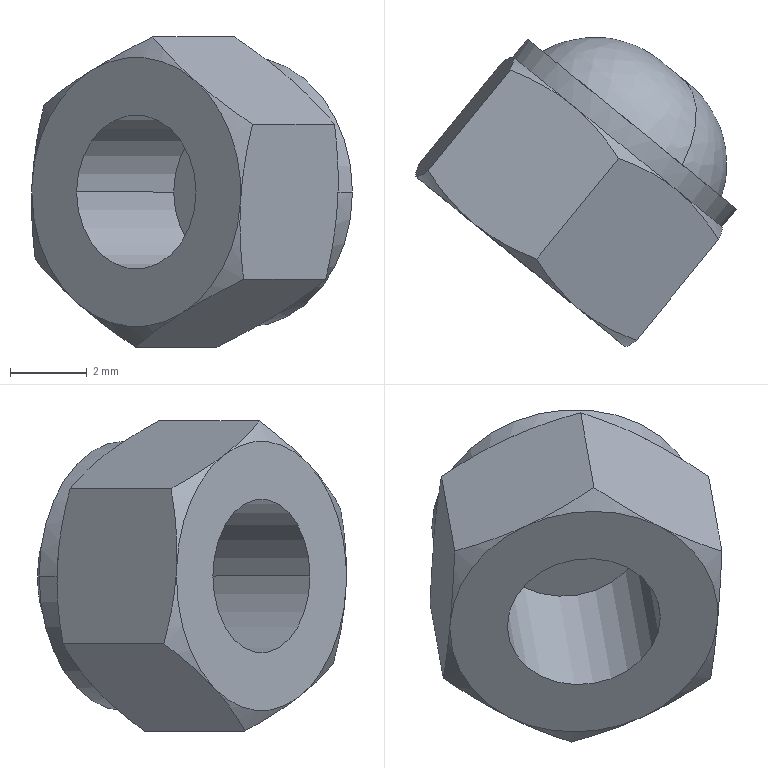Part | SolidWorks | features BaseBody 1 | 1 solid | 29 faces | box 8.341 x 8.038 x 8.061 mm | volume 172.858 mm3 | cone 14 | plane 9 | cylinder 4 | spline 2 | commonest cylinder face diameters 4 x2 7 x2
STEP:
#1=CARTESIAN_POINT('',(537.312,-141.656,258.325));
#2=VERTEX_POINT('',#1);
#3=CARTESIAN_POINT('',(534.695,-139.529,253.362));
#4=VERTEX_POINT('',#3);
#5=CARTESIAN_POINT('',(536.004,-140.592,255.843));
#6=DIRECTION('',(-0.6309,-0.7758,0.000000012));
#7=DIRECTION('',(0.7758,-0.6309,0.));
#8=AXIS2_PLACEMENT_3D('',#5,#6,#7);
#9=CIRCLE('',#8,3.);
#10=EDGE_CURVE('',#2,#4,#9,.T.);
#11=ORIENTED_EDGE('',*,*,#10,.F.);
#12=CARTESIAN_POINT('',(537.076,-139.274,255.843));
#13=VERTEX_POINT('',#12);
#14=CARTESIAN_POINT('',(535.614,-141.5,256.24));
#15=DIRECTION('',(-0.6417,0.5218,0.5621));
#16=DIRECTION('',(0.4361,-0.3546,0.8271));
#17=AXIS2_PLACEMENT_3D('',#14,#15,#16);
#18=CIRCLE('',#17,2.693);
#19=EDGE_CURVE('',#2,#13,#18,.T.);
#20=ORIENTED_EDGE('',*,*,#19,.T.);
#21=CARTESIAN_POINT('',(535.195,-141.159,255.446));
#22=DIRECTION('',(0.6417,-0.5218,-0.5621));
#23=DIRECTION('',(-0.4361,0.3546,-0.8271));
#24=AXIS2_PLACEMENT_3D('',#21,#22,#23);
#25=CIRCLE('',#24,2.693);
#26=EDGE_CURVE('',#4,#13,#25,.T.);
#27=ORIENTED_EDGE('',*,*,#26,.F.);
#28=EDGE_LOOP('',(#11,#20,#27));
#29=FACE_OUTER_BOUND('',#28,.T.);
#30=CARTESIAN_POINT('',(537.312,-141.656,258.325));
#31=CARTESIAN_POINT('',(533.462,-138.525,261.697));
#32=CARTESIAN_POINT('',(530.845,-136.398,256.735));
#33=CARTESIAN_POINT('',(534.695,-139.529,253.362));
#34=CARTESIAN_POINT('',(537.905,-140.499,257.928));
#35=CARTESIAN_POINT('',(534.671,-137.869,260.761));
#36=CARTESIAN_POINT('',(532.473,-136.081,256.592));
#37=CARTESIAN_POINT('',(535.707,-138.712,253.759));
#38=CARTESIAN_POINT('',(537.813,-139.56,256.95));
#39=CARTESIAN_POINT('',(536.096,-138.164,258.453));
#40=CARTESIAN_POINT('',(534.929,-137.215,256.241));
#41=CARTESIAN_POINT('',(536.646,-138.611,254.737));
#42=CARTESIAN_POINT('',(537.076,-139.274,255.843));
#43=CARTESIAN_POINT('',(537.076,-139.274,255.843));
#44=CARTESIAN_POINT('',(537.076,-139.274,255.843));
#45=CARTESIAN_POINT('',(537.076,-139.274,255.843));
#46=(BOUNDED_SURFACE()B_SPLINE_SURFACE(3,3,((#30,#31,#32,#33),(#34,#35,#36,#37),(#38,#39,#40,#41),(#42,#43,#44,#45)),.UNSPECIFIED.,.F.,.F.,.F.)B_SPLINE_SURFACE_WITH_KNOTS((4,4),(4,4),(0.,1.),(0.,1.),.UNSPECIFIED.)GEOMETRIC_REPRESENTATION_ITEM()RATIONAL_B_SPLINE_SURFACE(((1.,0.3333,0.3333,1.),(0.8455,0.2818,0.2818,0.8455),(0.8455,0.2818,0.2818,0.8455),(1.,0.3333,0.3333,1.)))REPRESENTATION_ITEM('')SURFACE());
#47=ADVANCED_FACE('',(#29),#46,.T.);
#48=CARTESIAN_POINT('',(534.074,-139.796,255.843));
#49=VERTEX_POINT('',#48);
#50=CARTESIAN_POINT('',(537.177,-142.32,255.843));
#51=VERTEX_POINT('',#50);
#52=CARTESIAN_POINT('',(535.625,-141.058,255.843));
#53=DIRECTION('',(-0.6309,-0.7758,0.000000012));
#54=DIRECTION('',(0.7758,-0.6309,0.));
#55=AXIS2_PLACEMENT_3D('',#52,#53,#54);
#56=CIRCLE('',#55,2.);
#57=EDGE_CURVE('',#49,#51,#56,.T.);
#58=ORIENTED_EDGE('',*,*,#57,.F.);
#59=CARTESIAN_POINT('',(531.55,-142.899,255.843));
#60=VERTEX_POINT('',#59);
#61=CARTESIAN_POINT('',(531.55,-142.899,255.843));
#62=DIRECTION('',(-0.6309,-0.7758,0.000000012));
#63=VECTOR('',#62,1000.);
#64=LINE('',#61,#63);
#65=EDGE_CURVE('',#49,#60,#64,.T.);
#66=ORIENTED_EDGE('',*,*,#65,.T.);
#67=CARTESIAN_POINT('',(534.653,-145.423,255.843));
#68=VERTEX_POINT('',#67);
#69=CARTESIAN_POINT('',(533.101,-144.161,255.843));
#70=DIRECTION('',(-0.6309,-0.7758,0.000000012));
#71=DIRECTION('',(0.7758,-0.6309,0.));
#72=AXIS2_PLACEMENT_3D('',#69,#70,#71);
#73=CIRCLE('',#72,2.);
#74=EDGE_CURVE('',#60,#68,#73,.T.);
#75=ORIENTED_EDGE('',*,*,#74,.T.);
#76=CARTESIAN_POINT('',(534.653,-145.423,255.843));
#77=DIRECTION('',(-0.6309,-0.7758,0.000000012));
#78=VECTOR('',#77,1000.);
#79=LINE('',#76,#78);
#80=EDGE_CURVE('',#51,#68,#79,.T.);
#81=ORIENTED_EDGE('',*,*,#80,.F.);
#82=EDGE_LOOP('',(#58,#66,#75,#81));
#83=FACE_OUTER_BOUND('',#82,.T.);
#84=CARTESIAN_POINT('',(533.101,-144.161,255.843));
#85=DIRECTION('',(-0.6309,-0.7758,0.000000012));
#86=DIRECTION('',(0.7758,-0.6309,0.));
#87=AXIS2_PLACEMENT_3D('',#84,#85,#86);
#88=CYLINDRICAL_SURFACE('',#87,2.);
#89=ADVANCED_FACE('',(#83),#88,.F.);
#90=CARTESIAN_POINT('',(531.575,-142.92,252.949));
#91=VERTEX_POINT('',#90);
#92=CARTESIAN_POINT('',(530.386,-141.953,255.843));
#93=VERTEX_POINT('',#92);
#94=CARTESIAN_POINT('',(533.101,-144.161,255.843));
#95=DIRECTION('',(0.6309,0.7758,-0.000000012));
#96=DIRECTION('',(-0.7758,0.6309,0.));
#97=AXIS2_PLACEMENT_3D('',#94,#95,#96);
#98=CIRCLE('',#97,3.5);
#99=EDGE_CURVE('',#91,#93,#98,.T.);
#100=ORIENTED_EDGE('',*,*,#99,.T.);
#101=CARTESIAN_POINT('',(530.382,-141.943,255.843));
#102=VERTEX_POINT('',#101);
#103=CARTESIAN_POINT('',(530.162,-141.365,255.843));
#104=DIRECTION('',(-0.3564,0.9343,-0.000000006));
#105=VECTOR('',#104,1000.);
#106=LINE('',#103,#105);
#107=EDGE_CURVE('',#93,#102,#106,.T.);
#108=ORIENTED_EDGE('',*,*,#107,.T.);
#109=CARTESIAN_POINT('',(530.476,-141.623,254.084));
#110=VERTEX_POINT('',#109);
#111=CARTESIAN_POINT('',(530.382,-141.943,255.843));
#112=CARTESIAN_POINT('',(530.364,-141.895,255.245));
#113=CARTESIAN_POINT('',(530.403,-141.779,254.661));
#114=CARTESIAN_POINT('',(530.476,-141.623,254.084));
#115=B_SPLINE_CURVE_WITH_KNOTS('',3,(#111,#112,#113,#114),.UNSPECIFIED.,.F.,.F.,(4,4),(0.0002548,0.002045),.UNSPECIFIED.);
#116=EDGE_CURVE('',#102,#110,#115,.T.);
#117=ORIENTED_EDGE('',*,*,#116,.T.);
#118=CARTESIAN_POINT('',(530.476,-141.623,254.084));
#119=CARTESIAN_POINT('',(530.779,-142.115,253.713));
#120=CARTESIAN_POINT('',(531.133,-142.56,253.336));
#121=CARTESIAN_POINT('',(531.575,-142.92,252.949));
#122=B_SPLINE_CURVE_WITH_KNOTS('',3,(#118,#119,#120,#121),.UNSPECIFIED.,.F.,.F.,(4,4),(0.,0.002045),.UNSPECIFIED.);
#123=EDGE_CURVE('',#110,#91,#122,.T.);
#124=ORIENTED_EDGE('',*,*,#123,.T.);
#125=EDGE_LOOP('',(#100,#108,#117,#124));
#126=FACE_OUTER_BOUND('',#125,.T.);
#127=CARTESIAN_POINT('',(533.3,-143.917,255.843));
#128=DIRECTION('',(0.6309,0.7758,-0.000000012));
#129=DIRECTION('',(-0.7758,0.6309,0.));
#130=AXIS2_PLACEMENT_3D('',#127,#128,#129);
#131=CONICAL_SURFACE('',#130,4.045,1.047);
#132=ADVANCED_FACE('',(#126),#131,.T.);
#133=CARTESIAN_POINT('',(538.333,-143.26,255.587));
#134=VERTEX_POINT('',#133);
#135=CARTESIAN_POINT('',(538.341,-143.266,255.843));
#136=VERTEX_POINT('',#135);
#137=CARTESIAN_POINT('',(535.625,-141.058,255.843));
#138=DIRECTION('',(-0.6309,-0.7758,0.000000012));
#139=DIRECTION('',(-0.4361,0.3546,-0.8271));
#140=AXIS2_PLACEMENT_3D('',#137,#138,#139);
#141=CIRCLE('',#140,3.5);
#142=EDGE_CURVE('',#134,#136,#141,.T.);
#143=ORIENTED_EDGE('',*,*,#142,.T.);
#144=CARTESIAN_POINT('',(538.344,-143.276,255.843));
#145=VERTEX_POINT('',#144);
#146=CARTESIAN_POINT('',(538.565,-143.854,255.843));
#147=DIRECTION('',(0.3564,-0.9343,0.000000006));
#148=VECTOR('',#147,1000.);
#149=LINE('',#146,#148);
#150=EDGE_CURVE('',#136,#145,#149,.T.);
#151=ORIENTED_EDGE('',*,*,#150,.T.);
#152=CARTESIAN_POINT('',(538.333,-143.26,255.587));
#153=CARTESIAN_POINT('',(538.338,-143.264,255.673));
#154=CARTESIAN_POINT('',(538.342,-143.27,255.758));
#155=CARTESIAN_POINT('',(538.344,-143.276,255.843));
#156=B_SPLINE_CURVE_WITH_KNOTS('',3,(#152,#153,#154,#155),.UNSPECIFIED.,.F.,.F.,(4,4),(0.,0.0002548),.UNSPECIFIED.);
#157=EDGE_CURVE('',#134,#145,#156,.T.);
#158=ORIENTED_EDGE('',*,*,#157,.F.);
#159=EDGE_LOOP('',(#143,#151,#158));
#160=FACE_OUTER_BOUND('',#159,.T.);
#161=CARTESIAN_POINT('',(535.427,-141.302,255.843));
#162=DIRECTION('',(-0.6309,-0.7758,0.000000012));
#163=DIRECTION('',(0.7758,-0.6309,0.));
#164=AXIS2_PLACEMENT_3D('',#161,#162,#163);
#165=CONICAL_SURFACE('',#164,4.045,1.047);
#166=ADVANCED_FACE('',(#160),#165,.T.);
#167=CARTESIAN_POINT('',(538.719,-142.801,255.843));
#168=VERTEX_POINT('',#167);
#169=CARTESIAN_POINT('',(533.288,-138.384,255.843));
#170=VERTEX_POINT('',#169);
#171=CARTESIAN_POINT('',(536.004,-140.592,255.843));
#172=DIRECTION('',(-0.6309,-0.7758,0.000000012));
#173=DIRECTION('',(0.7758,-0.6309,0.));
#174=AXIS2_PLACEMENT_3D('',#171,#172,#173);
#175=CIRCLE('',#174,3.5);
#176=EDGE_CURVE('',#168,#170,#175,.T.);
#177=ORIENTED_EDGE('',*,*,#176,.T.);
#178=CARTESIAN_POINT('',(532.91,-138.85,255.843));
#179=VERTEX_POINT('',#178);
#180=CARTESIAN_POINT('',(533.099,-138.617,255.843));
#181=DIRECTION('',(-0.6309,-0.7758,0.000000012));
#182=VECTOR('',#181,1000.);
#183=LINE('',#180,#182);
#184=EDGE_CURVE('',#170,#179,#183,.T.);
#185=ORIENTED_EDGE('',*,*,#184,.T.);
#186=CARTESIAN_POINT('',(532.917,-138.856,256.1));
#187=VERTEX_POINT('',#186);
#188=CARTESIAN_POINT('',(535.625,-141.058,255.843));
#189=DIRECTION('',(-0.6309,-0.7758,0.000000012));
#190=DIRECTION('',(-0.4361,0.3546,-0.8271));
#191=AXIS2_PLACEMENT_3D('',#188,#189,#190);
#192=CIRCLE('',#191,3.5);
#193=EDGE_CURVE('',#187,#179,#192,.T.);
#194=ORIENTED_EDGE('',*,*,#193,.F.);
#195=CARTESIAN_POINT('',(534.443,-140.097,258.994));
#196=VERTEX_POINT('',#195);
#197=CARTESIAN_POINT('',(535.625,-141.058,255.843));
#198=DIRECTION('',(-0.6309,-0.7758,0.000000012));
#199=DIRECTION('',(-0.4361,0.3546,-0.8271));
#200=AXIS2_PLACEMENT_3D('',#197,#198,#199);
#201=CIRCLE('',#200,3.5);
#202=EDGE_CURVE('',#196,#187,#201,.T.);
#203=ORIENTED_EDGE('',*,*,#202,.F.);
#204=CARTESIAN_POINT('',(537.151,-142.299,258.738));
#205=VERTEX_POINT('',#204);
#206=CARTESIAN_POINT('',(535.625,-141.058,255.843));
#207=DIRECTION('',(-0.6309,-0.7758,0.000000012));
#208=DIRECTION('',(-0.4361,0.3546,-0.8271));
#209=AXIS2_PLACEMENT_3D('',#206,#207,#208);
#210=CIRCLE('',#209,3.5);
#211=EDGE_CURVE('',#205,#196,#210,.T.);
#212=ORIENTED_EDGE('',*,*,#211,.F.);
#213=CARTESIAN_POINT('',(535.625,-141.058,255.843));
#214=DIRECTION('',(-0.6309,-0.7758,0.000000012));
#215=DIRECTION('',(-0.4361,0.3546,-0.8271));
#216=AXIS2_PLACEMENT_3D('',#213,#214,#215);
#217=CIRCLE('',#216,3.5);
#218=EDGE_CURVE('',#136,#205,#217,.T.);
#219=ORIENTED_EDGE('',*,*,#218,.F.);
#220=CARTESIAN_POINT('',(538.53,-143.033,255.843));
#221=DIRECTION('',(-0.6309,-0.7758,0.000000012));
#222=VECTOR('',#221,1000.);
#223=LINE('',#220,#222);
#224=EDGE_CURVE('',#168,#136,#223,.T.);
#225=ORIENTED_EDGE('',*,*,#224,.F.);
#226=EDGE_LOOP('',(#177,#185,#194,#203,#212,#219,#225));
#227=FACE_OUTER_BOUND('',#226,.T.);
#228=CARTESIAN_POINT('',(535.814,-140.825,255.843));
#229=DIRECTION('',(-0.6309,-0.7758,0.000000012));
#230=DIRECTION('',(0.7758,-0.6309,0.));
#231=AXIS2_PLACEMENT_3D('',#228,#229,#230);
#232=CYLINDRICAL_SURFACE('',#231,3.5);
#233=ADVANCED_FACE('',(#227),#232,.T.);
#234=CARTESIAN_POINT('',(533.101,-144.161,255.843));
#235=DIRECTION('',(-0.6309,-0.7758,0.000000012));
#236=DIRECTION('',(0.7758,-0.6309,0.));
#237=AXIS2_PLACEMENT_3D('',#234,#235,#236);
#238=CIRCLE('',#237,2.);
#239=EDGE_CURVE('',#68,#60,#238,.T.);
#240=ORIENTED_EDGE('',*,*,#239,.F.);
#241=ORIENTED_EDGE('',*,*,#74,.F.);
#242=EDGE_LOOP('',(#240,#241));
#243=FACE_BOUND('',#242,.T.);
#244=ORIENTED_EDGE('',*,*,#99,.F.);
#245=CARTESIAN_POINT('',(534.283,-145.122,252.692));
#246=VERTEX_POINT('',#245);
#247=CARTESIAN_POINT('',(533.101,-144.161,255.843));
#248=DIRECTION('',(0.6309,0.7758,-0.000000012));
#249=DIRECTION('',(-0.7758,0.6309,0.));
#250=AXIS2_PLACEMENT_3D('',#247,#248,#249);
#251=CIRCLE('',#250,3.5);
#252=EDGE_CURVE('',#246,#91,#251,.T.);
#253=ORIENTED_EDGE('',*,*,#252,.F.);
#254=CARTESIAN_POINT('',(535.81,-146.364,255.587));
#255=VERTEX_POINT('',#254);
#256=CARTESIAN_POINT('',(533.101,-144.161,255.843));
#257=DIRECTION('',(0.6309,0.7758,-0.000000012));
#258=DIRECTION('',(-0.7758,0.6309,0.));
#259=AXIS2_PLACEMENT_3D('',#256,#257,#258);
#260=CIRCLE('',#259,3.5);
#261=EDGE_CURVE('',#255,#246,#260,.T.);
#262=ORIENTED_EDGE('',*,*,#261,.F.);
#263=CARTESIAN_POINT('',(534.628,-145.403,258.738));
#264=VERTEX_POINT('',#263);
#265=CARTESIAN_POINT('',(533.101,-144.161,255.843));
#266=DIRECTION('',(0.6309,0.7758,-0.000000012));
#267=DIRECTION('',(-0.7758,0.6309,0.));
#268=AXIS2_PLACEMENT_3D('',#265,#266,#267);
#269=CIRCLE('',#268,3.5);
#270=EDGE_CURVE('',#264,#255,#269,.T.);
#271=ORIENTED_EDGE('',*,*,#270,.F.);
#272=CARTESIAN_POINT('',(531.92,-143.2,258.994));
#273=VERTEX_POINT('',#272);
#274=CARTESIAN_POINT('',(533.101,-144.161,255.843));
#275=DIRECTION('',(0.6309,0.7758,-0.000000012));
#276=DIRECTION('',(-0.7758,0.6309,0.));
#277=AXIS2_PLACEMENT_3D('',#274,#275,#276);
#278=CIRCLE('',#277,3.5);
#279=EDGE_CURVE('',#273,#264,#278,.T.);
#280=ORIENTED_EDGE('',*,*,#279,.F.);
#281=CARTESIAN_POINT('',(530.393,-141.959,256.1));
#282=VERTEX_POINT('',#281);
#283=CARTESIAN_POINT('',(533.101,-144.161,255.843));
#284=DIRECTION('',(0.6309,0.7758,-0.000000012));
#285=DIRECTION('',(-0.7758,0.6309,0.));
#286=AXIS2_PLACEMENT_3D('',#283,#284,#285);
#287=CIRCLE('',#286,3.5);
#288=EDGE_CURVE('',#282,#273,#287,.T.);
#289=ORIENTED_EDGE('',*,*,#288,.F.);
#290=CARTESIAN_POINT('',(533.101,-144.161,255.843));
#291=DIRECTION('',(0.6309,0.7758,-0.000000012));
#292=DIRECTION('',(-0.7758,0.6309,0.));
#293=AXIS2_PLACEMENT_3D('',#290,#291,#292);
#294=CIRCLE('',#293,3.5);
#295=EDGE_CURVE('',#93,#282,#294,.T.);
#296=ORIENTED_EDGE('',*,*,#295,.F.);
#297=EDGE_LOOP('',(#244,#253,#262,#271,#280,#289,#296));
#298=FACE_OUTER_BOUND('',#297,.T.);
#299=CARTESIAN_POINT('',(533.074,-144.139,255.792));
#300=DIRECTION('',(0.6309,0.7758,-0.000000012));
#301=DIRECTION('',(-0.7758,0.6309,0.));
#302=AXIS2_PLACEMENT_3D('',#299,#300,#301);
#303=PLANE('',#302);
#304=ADVANCED_FACE('',(#243,#298),#303,.F.);
#305=ORIENTED_EDGE('',*,*,#65,.F.);
#306=CARTESIAN_POINT('',(535.625,-141.058,255.843));
#307=DIRECTION('',(-0.6309,-0.7758,0.000000012));
#308=DIRECTION('',(0.7758,-0.6309,0.));
#309=AXIS2_PLACEMENT_3D('',#306,#307,#308);
#310=CIRCLE('',#309,2.);
#311=EDGE_CURVE('',#51,#49,#310,.T.);
#312=ORIENTED_EDGE('',*,*,#311,.F.);
#313=ORIENTED_EDGE('',*,*,#80,.T.);
#314=ORIENTED_EDGE('',*,*,#239,.T.);
#315=EDGE_LOOP('',(#305,#312,#313,#314));
#316=FACE_OUTER_BOUND('',#315,.T.);
#317=CARTESIAN_POINT('',(533.101,-144.161,255.843));
#318=DIRECTION('',(-0.6309,-0.7758,0.000000012));
#319=DIRECTION('',(0.7758,-0.6309,0.));
#320=AXIS2_PLACEMENT_3D('',#317,#318,#319);
#321=CYLINDRICAL_SURFACE('',#320,2.);
#322=ADVANCED_FACE('',(#316),#321,.F.);
#323=ORIENTED_EDGE('',*,*,#288,.T.);
#324=CARTESIAN_POINT('',(530.705,-141.81,258.115));
#325=VERTEX_POINT('',#324);
#326=CARTESIAN_POINT('',(531.92,-143.2,258.994));
#327=CARTESIAN_POINT('',(531.438,-142.808,258.694));
#328=CARTESIAN_POINT('',(531.046,-142.333,258.402));
#329=CARTESIAN_POINT('',(530.705,-141.81,258.115));
#330=B_SPLINE_CURVE_WITH_KNOTS('',3,(#326,#327,#328,#329),.UNSPECIFIED.,.F.,.F.,(4,4),(0.,0.002045),.UNSPECIFIED.);
#331=EDGE_CURVE('',#273,#325,#330,.T.);
#332=ORIENTED_EDGE('',*,*,#331,.T.);
#333=CARTESIAN_POINT('',(530.705,-141.81,258.115));
#334=CARTESIAN_POINT('',(530.548,-141.927,257.456));
#335=CARTESIAN_POINT('',(530.433,-141.991,256.787));
#336=CARTESIAN_POINT('',(530.393,-141.959,256.1));
#337=B_SPLINE_CURVE_WITH_KNOTS('',3,(#333,#334,#335,#336),.UNSPECIFIED.,.F.,.F.,(4,4),(0.,0.002045),.UNSPECIFIED.);
#338=EDGE_CURVE('',#325,#282,#337,.T.);
#339=ORIENTED_EDGE('',*,*,#338,.T.);
#340=EDGE_LOOP('',(#323,#332,#339));
#341=FACE_OUTER_BOUND('',#340,.T.);
#342=CARTESIAN_POINT('',(533.3,-143.917,255.843));
#343=DIRECTION('',(0.6309,0.7758,-0.000000012));
#344=DIRECTION('',(-0.7758,0.6309,0.));
#345=AXIS2_PLACEMENT_3D('',#342,#343,#344);
#346=CONICAL_SURFACE('',#345,4.045,1.047);
#347=ADVANCED_FACE('',(#341),#346,.T.);
#348=ORIENTED_EDGE('',*,*,#107,.F.);
#349=ORIENTED_EDGE('',*,*,#295,.T.);
#350=CARTESIAN_POINT('',(530.393,-141.959,256.1));
#351=CARTESIAN_POINT('',(530.388,-141.955,256.014));
#352=CARTESIAN_POINT('',(530.385,-141.95,255.928));
#353=CARTESIAN_POINT('',(530.382,-141.943,255.843));
#354=B_SPLINE_CURVE_WITH_KNOTS('',3,(#350,#351,#352,#353),.UNSPECIFIED.,.F.,.F.,(4,4),(0.,0.0002548),.UNSPECIFIED.);
#355=EDGE_CURVE('',#282,#102,#354,.T.);
#356=ORIENTED_EDGE('',*,*,#355,.T.);
#357=EDGE_LOOP('',(#348,#349,#356));
#358=FACE_OUTER_BOUND('',#357,.T.);
#359=CARTESIAN_POINT('',(533.3,-143.917,255.843));
#360=DIRECTION('',(0.6309,0.7758,-0.000000012));
#361=DIRECTION('',(-0.7758,0.6309,0.));
#362=AXIS2_PLACEMENT_3D('',#359,#360,#361);
#363=CONICAL_SURFACE('',#362,4.045,1.047);
#364=ADVANCED_FACE('',(#358),#363,.T.);
#365=ORIENTED_EDGE('',*,*,#252,.T.);
#366=CARTESIAN_POINT('',(533.069,-143.732,251.813));
#367=VERTEX_POINT('',#366);
#368=CARTESIAN_POINT('',(531.575,-142.92,252.949));
#369=CARTESIAN_POINT('',(532.018,-143.28,252.561));
#370=CARTESIAN_POINT('',(532.525,-143.535,252.184));
#371=CARTESIAN_POINT('',(533.069,-143.732,251.813));
#372=B_SPLINE_CURVE_WITH_KNOTS('',3,(#368,#369,#370,#371),.UNSPECIFIED.,.F.,.F.,(4,4),(0.,0.002045),.UNSPECIFIED.);
#373=EDGE_CURVE('',#91,#367,#372,.T.);
#374=ORIENTED_EDGE('',*,*,#373,.T.);
#375=CARTESIAN_POINT('',(533.069,-143.732,251.813));
#376=CARTESIAN_POINT('',(533.41,-144.255,252.1));
#377=CARTESIAN_POINT('',(533.802,-144.731,252.392));
#378=CARTESIAN_POINT('',(534.283,-145.122,252.692));
#379=B_SPLINE_CURVE_WITH_KNOTS('',3,(#375,#376,#377,#378),.UNSPECIFIED.,.F.,.F.,(4,4),(0.,0.002045),.UNSPECIFIED.);
#380=EDGE_CURVE('',#367,#246,#379,.T.);
#381=ORIENTED_EDGE('',*,*,#380,.T.);
#382=EDGE_LOOP('',(#365,#374,#381));
#383=FACE_OUTER_BOUND('',#382,.T.);
#384=CARTESIAN_POINT('',(533.3,-143.917,255.843));
#385=DIRECTION('',(0.6309,0.7758,-0.000000012));
#386=DIRECTION('',(-0.7758,0.6309,0.));
#387=AXIS2_PLACEMENT_3D('',#384,#385,#386);
#388=CONICAL_SURFACE('',#387,4.045,1.047);
#389=ADVANCED_FACE('',(#383),#388,.T.);
#390=ORIENTED_EDGE('',*,*,#261,.T.);
#391=CARTESIAN_POINT('',(535.892,-146.028,253.572));
#392=VERTEX_POINT('',#391);
#393=CARTESIAN_POINT('',(534.283,-145.122,252.692));
#394=CARTESIAN_POINT('',(534.765,-145.514,252.992));
#395=CARTESIAN_POINT('',(535.311,-145.801,253.284));
#396=CARTESIAN_POINT('',(535.892,-146.028,253.572));
#397=B_SPLINE_CURVE_WITH_KNOTS('',3,(#393,#394,#395,#396),.UNSPECIFIED.,.F.,.F.,(4,4),(0.,0.002045),.UNSPECIFIED.);
#398=EDGE_CURVE('',#246,#392,#397,.T.);
#399=ORIENTED_EDGE('',*,*,#398,.T.);
#400=CARTESIAN_POINT('',(535.892,-146.028,253.572));
#401=CARTESIAN_POINT('',(535.809,-146.206,254.23));
#402=CARTESIAN_POINT('',(535.77,-146.332,254.899));
#403=CARTESIAN_POINT('',(535.81,-146.364,255.587));
#404=B_SPLINE_CURVE_WITH_KNOTS('',3,(#400,#401,#402,#403),.UNSPECIFIED.,.F.,.F.,(4,4),(0.,0.002045),.UNSPECIFIED.);
#405=EDGE_CURVE('',#392,#255,#404,.T.);
#406=ORIENTED_EDGE('',*,*,#405,.T.);
#407=EDGE_LOOP('',(#390,#399,#406));
#408=FACE_OUTER_BOUND('',#407,.T.);
#409=CARTESIAN_POINT('',(533.3,-143.917,255.843));
#410=DIRECTION('',(0.6309,0.7758,-0.000000012));
#411=DIRECTION('',(-0.7758,0.6309,0.));
#412=AXIS2_PLACEMENT_3D('',#409,#410,#411);
#413=CONICAL_SURFACE('',#412,4.045,1.047);
#414=ADVANCED_FACE('',(#408),#413,.T.);
#415=CARTESIAN_POINT('',(536.122,-146.214,257.602));
#416=VERTEX_POINT('',#415);
#417=CARTESIAN_POINT('',(536.122,-146.214,257.602));
#418=CARTESIAN_POINT('',(535.578,-146.018,257.973));
#419=CARTESIAN_POINT('',(535.07,-145.762,258.35));
#420=CARTESIAN_POINT('',(534.628,-145.403,258.738));
#421=B_SPLINE_CURVE_WITH_KNOTS('',3,(#417,#418,#419,#420),.UNSPECIFIED.,.F.,.F.,(4,4),(0.,0.002045),.UNSPECIFIED.);
#422=EDGE_CURVE('',#416,#264,#421,.T.);
#423=ORIENTED_EDGE('',*,*,#422,.T.);
#424=ORIENTED_EDGE('',*,*,#270,.T.);
#425=CARTESIAN_POINT('',(535.81,-146.364,255.587));
#426=CARTESIAN_POINT('',(535.849,-146.395,256.275));
#427=CARTESIAN_POINT('',(535.964,-146.332,256.944));
#428=CARTESIAN_POINT('',(536.122,-146.214,257.602));
#429=B_SPLINE_CURVE_WITH_KNOTS('',3,(#425,#426,#427,#428),.UNSPECIFIED.,.F.,.F.,(4,4),(0.,0.002045),.UNSPECIFIED.);
#430=EDGE_CURVE('',#255,#416,#429,.T.);
#431=ORIENTED_EDGE('',*,*,#430,.T.);
#432=EDGE_LOOP('',(#423,#424,#431));
#433=FACE_OUTER_BOUND('',#432,.T.);
#434=CARTESIAN_POINT('',(533.3,-143.917,255.843));
#435=DIRECTION('',(0.6309,0.7758,-0.000000012));
#436=DIRECTION('',(-0.7758,0.6309,0.));
#437=AXIS2_PLACEMENT_3D('',#434,#435,#436);
#438=CONICAL_SURFACE('',#437,4.045,1.047);
#439=ADVANCED_FACE('',(#433),#438,.T.);
#440=CARTESIAN_POINT('',(533.528,-144.106,259.874));
#441=VERTEX_POINT('',#440);
#442=CARTESIAN_POINT('',(533.528,-144.106,259.874));
#443=CARTESIAN_POINT('',(532.947,-143.878,259.587));
#444=CARTESIAN_POINT('',(532.401,-143.592,259.295));
#445=CARTESIAN_POINT('',(531.92,-143.2,258.994));
#446=B_SPLINE_CURVE_WITH_KNOTS('',3,(#442,#443,#444,#445),.UNSPECIFIED.,.F.,.F.,(4,4),(0.,0.002045),.UNSPECIFIED.);
#447=EDGE_CURVE('',#441,#273,#446,.T.);
#448=ORIENTED_EDGE('',*,*,#447,.T.);
#449=ORIENTED_EDGE('',*,*,#279,.T.);
#450=CARTESIAN_POINT('',(534.628,-145.403,258.738));
#451=CARTESIAN_POINT('',(534.185,-145.043,259.126));
#452=CARTESIAN_POINT('',(533.832,-144.598,259.503));
#453=CARTESIAN_POINT('',(533.528,-144.106,259.874));
#454=B_SPLINE_CURVE_WITH_KNOTS('',3,(#450,#451,#452,#453),.UNSPECIFIED.,.F.,.F.,(4,4),(0.,0.002045),.UNSPECIFIED.);
#455=EDGE_CURVE('',#264,#441,#454,.T.);
#456=ORIENTED_EDGE('',*,*,#455,.T.);
#457=EDGE_LOOP('',(#448,#449,#456));
#458=FACE_OUTER_BOUND('',#457,.T.);
#459=CARTESIAN_POINT('',(533.3,-143.917,255.843));
#460=DIRECTION('',(0.6309,0.7758,-0.000000012));
#461=DIRECTION('',(-0.7758,0.6309,0.));
#462=AXIS2_PLACEMENT_3D('',#459,#460,#461);
#463=CONICAL_SURFACE('',#462,4.045,1.047);
#464=ADVANCED_FACE('',(#458),#463,.T.);
#465=ORIENTED_EDGE('',*,*,#311,.T.);
#466=ORIENTED_EDGE('',*,*,#57,.T.);
#467=EDGE_LOOP('',(#465,#466));
#468=FACE_OUTER_BOUND('',#467,.T.);
#469=CARTESIAN_POINT('',(534.862,-140.437,254.396));
#470=DIRECTION('',(-0.6309,-0.7758,0.000000012));
#471=DIRECTION('',(0.7758,-0.6309,0.));
#472=AXIS2_PLACEMENT_3D('',#469,#470,#471);
#473=PLANE('',#472);
#474=ADVANCED_FACE('',(#468),#473,.T.);
#475=CARTESIAN_POINT('',(535.658,-141.487,259.874));
#476=VERTEX_POINT('',#475);
#477=CARTESIAN_POINT('',(533.528,-144.106,259.874));
#478=DIRECTION('',(0.6309,0.7758,-0.000000012));
#479=VECTOR('',#478,1000.);
#480=LINE('',#477,#479);
#481=EDGE_CURVE('',#441,#476,#480,.T.);
#482=ORIENTED_EDGE('',*,*,#481,.T.);
#483=CARTESIAN_POINT('',(535.658,-141.487,259.874));
#484=CARTESIAN_POINT('',(535.317,-140.964,259.587));
#485=CARTESIAN_POINT('',(534.925,-140.489,259.295));
#486=CARTESIAN_POINT('',(534.443,-140.097,258.994));
#487=B_SPLINE_CURVE_WITH_KNOTS('',3,(#483,#484,#485,#486),.UNSPECIFIED.,.F.,.F.,(4,4),(0.,0.002045),.UNSPECIFIED.);
#488=EDGE_CURVE('',#476,#196,#487,.T.);
#489=ORIENTED_EDGE('',*,*,#488,.T.);
#490=CARTESIAN_POINT('',(532.835,-139.192,258.115));
#491=VERTEX_POINT('',#490);
#492=CARTESIAN_POINT('',(534.443,-140.097,258.994));
#493=CARTESIAN_POINT('',(533.962,-139.705,258.694));
#494=CARTESIAN_POINT('',(533.416,-139.419,258.402));
#495=CARTESIAN_POINT('',(532.835,-139.192,258.115));
#496=B_SPLINE_CURVE_WITH_KNOTS('',3,(#492,#493,#494,#495),.UNSPECIFIED.,.F.,.F.,(4,4),(0.,0.002045),.UNSPECIFIED.);
#497=EDGE_CURVE('',#196,#491,#496,.T.);
#498=ORIENTED_EDGE('',*,*,#497,.T.);
#499=CARTESIAN_POINT('',(532.835,-139.192,258.115));
#500=DIRECTION('',(-0.6309,-0.7758,0.000000012));
#501=VECTOR('',#500,1000.);
#502=LINE('',#499,#501);
#503=EDGE_CURVE('',#491,#325,#502,.T.);
#504=ORIENTED_EDGE('',*,*,#503,.T.);
#505=ORIENTED_EDGE('',*,*,#331,.F.);
#506=ORIENTED_EDGE('',*,*,#447,.F.);
#507=EDGE_LOOP('',(#482,#489,#498,#504,#505,#506));
#508=FACE_OUTER_BOUND('',#507,.T.);
#509=CARTESIAN_POINT('',(533.331,-144.348,259.874));
#510=DIRECTION('',(-0.3377,0.2746,0.9003));
#511=DIRECTION('',(0.9363,0.,0.3512));
#512=AXIS2_PLACEMENT_3D('',#509,#510,#511);
#513=PLANE('',#512);
#514=ADVANCED_FACE('',(#508),#513,.T.);
#515=ORIENTED_EDGE('',*,*,#503,.F.);
#516=CARTESIAN_POINT('',(532.835,-139.192,258.115));
#517=CARTESIAN_POINT('',(532.917,-139.013,257.456));
#518=CARTESIAN_POINT('',(532.956,-138.887,256.787));
#519=CARTESIAN_POINT('',(532.917,-138.856,256.1));
#520=B_SPLINE_CURVE_WITH_KNOTS('',3,(#516,#517,#518,#519),.UNSPECIFIED.,.F.,.F.,(4,4),(0.,0.002045),.UNSPECIFIED.);
#521=EDGE_CURVE('',#491,#187,#520,.T.);
#522=ORIENTED_EDGE('',*,*,#521,.T.);
#523=CARTESIAN_POINT('',(532.605,-139.005,254.084));
#524=VERTEX_POINT('',#523);
#525=CARTESIAN_POINT('',(532.917,-138.856,256.1));
#526=CARTESIAN_POINT('',(532.878,-138.824,255.412));
#527=CARTESIAN_POINT('',(532.763,-138.887,254.743));
#528=CARTESIAN_POINT('',(532.605,-139.005,254.084));
#529=B_SPLINE_CURVE_WITH_KNOTS('',3,(#525,#526,#527,#528),.UNSPECIFIED.,.F.,.F.,(4,4),(0.,0.002045),.UNSPECIFIED.);
#530=EDGE_CURVE('',#187,#524,#529,.T.);
#531=ORIENTED_EDGE('',*,*,#530,.T.);
#532=CARTESIAN_POINT('',(530.278,-141.866,254.084));
#533=DIRECTION('',(-0.6309,-0.7758,0.));
#534=VECTOR('',#533,1000.);
#535=LINE('',#532,#534);
#536=EDGE_CURVE('',#524,#110,#535,.T.);
#537=ORIENTED_EDGE('',*,*,#536,.T.);
#538=ORIENTED_EDGE('',*,*,#116,.F.);
#539=ORIENTED_EDGE('',*,*,#355,.F.);
#540=ORIENTED_EDGE('',*,*,#338,.F.);
#541=EDGE_LOOP('',(#515,#522,#531,#537,#538,#539,#540));
#542=FACE_OUTER_BOUND('',#541,.T.);
#543=CARTESIAN_POINT('',(530.508,-142.052,258.115));
#544=DIRECTION('',(-0.7738,0.6292,0.07324));
#545=DIRECTION('',(-0.6309,-0.7758,0.));
#546=AXIS2_PLACEMENT_3D('',#543,#544,#545);
#547=PLANE('',#546);
#548=ADVANCED_FACE('',(#542),#547,.T.);
#549=ORIENTED_EDGE('',*,*,#123,.F.);
#550=ORIENTED_EDGE('',*,*,#536,.F.);
#551=CARTESIAN_POINT('',(534.099,-139.817,252.949));
#552=VERTEX_POINT('',#551);
#553=CARTESIAN_POINT('',(532.605,-139.005,254.084));
#554=CARTESIAN_POINT('',(533.149,-139.201,253.713));
#555=CARTESIAN_POINT('',(533.656,-139.457,253.336));
#556=CARTESIAN_POINT('',(534.099,-139.817,252.949));
#557=B_SPLINE_CURVE_WITH_KNOTS('',3,(#553,#554,#555,#556),.UNSPECIFIED.,.F.,.F.,(4,4),(0.,0.002045),.UNSPECIFIED.);
#558=EDGE_CURVE('',#524,#552,#557,.T.);
#559=ORIENTED_EDGE('',*,*,#558,.T.);
#560=CARTESIAN_POINT('',(535.198,-141.114,251.813));
#561=VERTEX_POINT('',#560);
#562=CARTESIAN_POINT('',(534.099,-139.817,252.949));
#563=CARTESIAN_POINT('',(534.541,-140.177,252.561));
#564=CARTESIAN_POINT('',(534.895,-140.621,252.184));
#565=CARTESIAN_POINT('',(535.198,-141.114,251.813));
#566=B_SPLINE_CURVE_WITH_KNOTS('',3,(#562,#563,#564,#565),.UNSPECIFIED.,.F.,.F.,(4,4),(0.,0.002045),.UNSPECIFIED.);
#567=EDGE_CURVE('',#552,#561,#566,.T.);
#568=ORIENTED_EDGE('',*,*,#567,.T.);
#569=CARTESIAN_POINT('',(535.198,-141.114,251.813));
#570=DIRECTION('',(-0.6309,-0.7758,0.000000012));
#571=VECTOR('',#570,1000.);
#572=LINE('',#569,#571);
#573=EDGE_CURVE('',#561,#367,#572,.T.);
#574=ORIENTED_EDGE('',*,*,#573,.T.);
#575=ORIENTED_EDGE('',*,*,#373,.F.);
#576=EDGE_LOOP('',(#549,#550,#559,#568,#574,#575));
#577=FACE_OUTER_BOUND('',#576,.T.);
#578=CARTESIAN_POINT('',(530.278,-141.866,254.084));
#579=DIRECTION('',(-0.4361,0.3546,-0.8271));
#580=DIRECTION('',(-0.8846,0.,0.4664));
#581=AXIS2_PLACEMENT_3D('',#578,#579,#580);
#582=PLANE('',#581);
#583=ADVANCED_FACE('',(#577),#582,.T.);
#584=ORIENTED_EDGE('',*,*,#380,.F.);
#585=ORIENTED_EDGE('',*,*,#573,.F.);
#586=CARTESIAN_POINT('',(536.807,-142.019,252.692));
#587=VERTEX_POINT('',#586);
#588=CARTESIAN_POINT('',(535.198,-141.114,251.813));
#589=CARTESIAN_POINT('',(535.78,-141.341,252.1));
#590=CARTESIAN_POINT('',(536.325,-141.627,252.392));
#591=CARTESIAN_POINT('',(536.807,-142.019,252.692));
#592=B_SPLINE_CURVE_WITH_KNOTS('',3,(#588,#589,#590,#591),.UNSPECIFIED.,.F.,.F.,(4,4),(0.,0.002045),.UNSPECIFIED.);
#593=EDGE_CURVE('',#561,#587,#592,.T.);
#594=ORIENTED_EDGE('',*,*,#593,.T.);
#595=CARTESIAN_POINT('',(538.021,-143.409,253.572));
#596=VERTEX_POINT('',#595);
#597=CARTESIAN_POINT('',(536.807,-142.019,252.692));
#598=CARTESIAN_POINT('',(537.289,-142.411,252.992));
#599=CARTESIAN_POINT('',(537.68,-142.887,253.284));
#600=CARTESIAN_POINT('',(538.021,-143.409,253.572));
#601=B_SPLINE_CURVE_WITH_KNOTS('',3,(#597,#598,#599,#600),.UNSPECIFIED.,.F.,.F.,(4,4),(0.,0.002045),.UNSPECIFIED.);
#602=EDGE_CURVE('',#587,#596,#601,.T.);
#603=ORIENTED_EDGE('',*,*,#602,.T.);
#604=CARTESIAN_POINT('',(538.021,-143.409,253.572));
#605=DIRECTION('',(-0.6309,-0.7758,0.000000012));
#606=VECTOR('',#605,1000.);
#607=LINE('',#604,#606);
#608=EDGE_CURVE('',#596,#392,#607,.T.);
#609=ORIENTED_EDGE('',*,*,#608,.T.);
#610=ORIENTED_EDGE('',*,*,#398,.F.);
#611=EDGE_LOOP('',(#584,#585,#594,#603,#609,#610));
#612=FACE_OUTER_BOUND('',#611,.T.);
#613=CARTESIAN_POINT('',(532.872,-143.975,251.813));
#614=DIRECTION('',(0.3377,-0.2746,-0.9003));
#615=DIRECTION('',(-0.9363,0.,-0.3512));
#616=AXIS2_PLACEMENT_3D('',#613,#614,#615);
#617=PLANE('',#616);
#618=ADVANCED_FACE('',(#612),#617,.T.);
#619=ORIENTED_EDGE('',*,*,#405,.F.);
#620=ORIENTED_EDGE('',*,*,#608,.F.);
#621=CARTESIAN_POINT('',(538.021,-143.409,253.572));
#622=CARTESIAN_POINT('',(538.179,-143.292,254.23));
#623=CARTESIAN_POINT('',(538.294,-143.228,254.899));
#624=CARTESIAN_POINT('',(538.333,-143.26,255.587));
#625=B_SPLINE_CURVE_WITH_KNOTS('',3,(#621,#622,#623,#624),.UNSPECIFIED.,.F.,.F.,(4,4),(0.,0.002045),.UNSPECIFIED.);
#626=EDGE_CURVE('',#596,#134,#625,.T.);
#627=ORIENTED_EDGE('',*,*,#626,.T.);
#628=ORIENTED_EDGE('',*,*,#157,.T.);
#629=CARTESIAN_POINT('',(538.251,-143.596,257.602));
#630=VERTEX_POINT('',#629);
#631=CARTESIAN_POINT('',(538.344,-143.276,255.843));
#632=CARTESIAN_POINT('',(538.363,-143.324,256.442));
#633=CARTESIAN_POINT('',(538.323,-143.44,257.026));
#634=CARTESIAN_POINT('',(538.251,-143.596,257.602));
#635=B_SPLINE_CURVE_WITH_KNOTS('',3,(#631,#632,#633,#634),.UNSPECIFIED.,.F.,.F.,(4,4),(0.0002548,0.002045),.UNSPECIFIED.);
#636=EDGE_CURVE('',#145,#630,#635,.T.);
#637=ORIENTED_EDGE('',*,*,#636,.T.);
#638=CARTESIAN_POINT('',(535.924,-146.457,257.602));
#639=DIRECTION('',(-0.6309,-0.7758,0.));
#640=VECTOR('',#639,1000.);
#641=LINE('',#638,#640);
#642=EDGE_CURVE('',#630,#416,#641,.T.);
#643=ORIENTED_EDGE('',*,*,#642,.T.);
#644=ORIENTED_EDGE('',*,*,#430,.F.);
#645=EDGE_LOOP('',(#619,#620,#627,#628,#637,#643,#644));
#646=FACE_OUTER_BOUND('',#645,.T.);
#647=CARTESIAN_POINT('',(535.695,-146.27,253.572));
#648=DIRECTION('',(0.7738,-0.6292,-0.07324));
#649=DIRECTION('',(0.6309,0.7758,0.));
#650=AXIS2_PLACEMENT_3D('',#647,#648,#649);
#651=PLANE('',#650);
#652=ADVANCED_FACE('',(#646),#651,.T.);
#653=ORIENTED_EDGE('',*,*,#642,.F.);
#654=CARTESIAN_POINT('',(538.251,-143.596,257.602));
#655=CARTESIAN_POINT('',(537.948,-143.104,257.973));
#656=CARTESIAN_POINT('',(537.594,-142.659,258.35));
#657=CARTESIAN_POINT('',(537.151,-142.299,258.738));
#658=B_SPLINE_CURVE_WITH_KNOTS('',3,(#654,#655,#656,#657),.UNSPECIFIED.,.F.,.F.,(4,4),(0.,0.002045),.UNSPECIFIED.);
#659=EDGE_CURVE('',#630,#205,#658,.T.);
#660=ORIENTED_EDGE('',*,*,#659,.T.);
#661=CARTESIAN_POINT('',(537.151,-142.299,258.738));
#662=CARTESIAN_POINT('',(536.709,-141.939,259.126));
#663=CARTESIAN_POINT('',(536.201,-141.684,259.503));
#664=CARTESIAN_POINT('',(535.658,-141.487,259.874));
#665=B_SPLINE_CURVE_WITH_KNOTS('',3,(#661,#662,#663,#664),.UNSPECIFIED.,.F.,.F.,(4,4),(0.,0.002045),.UNSPECIFIED.);
#666=EDGE_CURVE('',#205,#476,#665,.T.);
#667=ORIENTED_EDGE('',*,*,#666,.T.);
#668=ORIENTED_EDGE('',*,*,#481,.F.);
#669=ORIENTED_EDGE('',*,*,#455,.F.);
#670=ORIENTED_EDGE('',*,*,#422,.F.);
#671=EDGE_LOOP('',(#653,#660,#667,#668,#669,#670));
#672=FACE_OUTER_BOUND('',#671,.T.);
#673=CARTESIAN_POINT('',(535.924,-146.457,257.602));
#674=DIRECTION('',(0.4361,-0.3546,0.8271));
#675=DIRECTION('',(0.8846,0.,-0.4664));
#676=AXIS2_PLACEMENT_3D('',#673,#674,#675);
#677=PLANE('',#676);
#678=ADVANCED_FACE('',(#672),#677,.T.);
#679=ORIENTED_EDGE('',*,*,#666,.F.);
#680=ORIENTED_EDGE('',*,*,#211,.T.);
#681=ORIENTED_EDGE('',*,*,#488,.F.);
#682=EDGE_LOOP('',(#679,#680,#681));
#683=FACE_OUTER_BOUND('',#682,.T.);
#684=CARTESIAN_POINT('',(535.427,-141.302,255.843));
#685=DIRECTION('',(-0.6309,-0.7758,0.000000012));
#686=DIRECTION('',(0.7758,-0.6309,0.));
#687=AXIS2_PLACEMENT_3D('',#684,#685,#686);
#688=CONICAL_SURFACE('',#687,4.045,1.047);
#689=ADVANCED_FACE('',(#683),#688,.T.);
#690=ORIENTED_EDGE('',*,*,#497,.F.);
#691=ORIENTED_EDGE('',*,*,#202,.T.);
#692=ORIENTED_EDGE('',*,*,#521,.F.);
#693=EDGE_LOOP('',(#690,#691,#692));
#694=FACE_OUTER_BOUND('',#693,.T.);
#695=CARTESIAN_POINT('',(535.427,-141.302,255.843));
#696=DIRECTION('',(-0.6309,-0.7758,0.000000012));
#697=DIRECTION('',(0.7758,-0.6309,0.));
#698=AXIS2_PLACEMENT_3D('',#695,#696,#697);
#699=CONICAL_SURFACE('',#698,4.045,1.047);
#700=ADVANCED_FACE('',(#694),#699,.T.);
#701=ORIENTED_EDGE('',*,*,#530,.F.);
#702=ORIENTED_EDGE('',*,*,#193,.T.);
#703=CARTESIAN_POINT('',(535.625,-141.058,255.843));
#704=DIRECTION('',(-0.6309,-0.7758,0.000000012));
#705=DIRECTION('',(-0.4361,0.3546,-0.8271));
#706=AXIS2_PLACEMENT_3D('',#703,#704,#705);
#707=CIRCLE('',#706,3.5);
#708=EDGE_CURVE('',#179,#552,#707,.T.);
#709=ORIENTED_EDGE('',*,*,#708,.T.);
#710=ORIENTED_EDGE('',*,*,#558,.F.);
#711=EDGE_LOOP('',(#701,#702,#709,#710));
#712=FACE_OUTER_BOUND('',#711,.T.);
#713=CARTESIAN_POINT('',(535.427,-141.302,255.843));
#714=DIRECTION('',(-0.6309,-0.7758,0.000000012));
#715=DIRECTION('',(0.7758,-0.6309,0.));
#716=AXIS2_PLACEMENT_3D('',#713,#714,#715);
#717=CONICAL_SURFACE('',#716,4.045,1.047);
#718=ADVANCED_FACE('',(#712),#717,.T.);
#719=CARTESIAN_POINT('',(535.625,-141.058,255.843));
#720=DIRECTION('',(-0.6309,-0.7758,0.000000012));
#721=DIRECTION('',(-0.4361,0.3546,-0.8271));
#722=AXIS2_PLACEMENT_3D('',#719,#720,#721);
#723=CIRCLE('',#722,3.5);
#724=EDGE_CURVE('',#552,#587,#723,.T.);
#725=ORIENTED_EDGE('',*,*,#724,.T.);
#726=ORIENTED_EDGE('',*,*,#593,.F.);
#727=ORIENTED_EDGE('',*,*,#567,.F.);
#728=EDGE_LOOP('',(#725,#726,#727));
#729=FACE_OUTER_BOUND('',#728,.T.);
#730=CARTESIAN_POINT('',(535.427,-141.302,255.843));
#731=DIRECTION('',(-0.6309,-0.7758,0.000000012));
#732=DIRECTION('',(0.7758,-0.6309,0.));
#733=AXIS2_PLACEMENT_3D('',#730,#731,#732);
#734=CONICAL_SURFACE('',#733,4.045,1.047);
#735=ADVANCED_FACE('',(#729),#734,.T.);
#736=CARTESIAN_POINT('',(535.625,-141.058,255.843));
#737=DIRECTION('',(-0.6309,-0.7758,0.000000012));
#738=DIRECTION('',(-0.4361,0.3546,-0.8271));
#739=AXIS2_PLACEMENT_3D('',#736,#737,#738);
#740=CIRCLE('',#739,3.5);
#741=EDGE_CURVE('',#587,#134,#740,.T.);
#742=ORIENTED_EDGE('',*,*,#741,.T.);
#743=ORIENTED_EDGE('',*,*,#626,.F.);
#744=ORIENTED_EDGE('',*,*,#602,.F.);
#745=EDGE_LOOP('',(#742,#743,#744));
#746=FACE_OUTER_BOUND('',#745,.T.);
#747=CARTESIAN_POINT('',(535.427,-141.302,255.843));
#748=DIRECTION('',(-0.6309,-0.7758,0.000000012));
#749=DIRECTION('',(0.7758,-0.6309,0.));
#750=AXIS2_PLACEMENT_3D('',#747,#748,#749);
#751=CONICAL_SURFACE('',#750,4.045,1.047);
#752=ADVANCED_FACE('',(#746),#751,.T.);
#753=ORIENTED_EDGE('',*,*,#150,.F.);
#754=ORIENTED_EDGE('',*,*,#218,.T.);
#755=ORIENTED_EDGE('',*,*,#659,.F.);
#756=ORIENTED_EDGE('',*,*,#636,.F.);
#757=EDGE_LOOP('',(#753,#754,#755,#756));
#758=FACE_OUTER_BOUND('',#757,.T.);
#759=CARTESIAN_POINT('',(535.427,-141.302,255.843));
#760=DIRECTION('',(-0.6309,-0.7758,0.000000012));
#761=DIRECTION('',(0.7758,-0.6309,0.));
#762=AXIS2_PLACEMENT_3D('',#759,#760,#761);
#763=CONICAL_SURFACE('',#762,4.045,1.047);
#764=ADVANCED_FACE('',(#758),#763,.T.);
#765=ORIENTED_EDGE('',*,*,#184,.F.);
#766=CARTESIAN_POINT('',(536.004,-140.592,255.843));
#767=DIRECTION('',(-0.6309,-0.7758,0.000000012));
#768=DIRECTION('',(0.7758,-0.6309,0.));
#769=AXIS2_PLACEMENT_3D('',#766,#767,#768);
#770=CIRCLE('',#769,3.5);
#771=EDGE_CURVE('',#170,#168,#770,.T.);
#772=ORIENTED_EDGE('',*,*,#771,.T.);
#773=ORIENTED_EDGE('',*,*,#224,.T.);
#774=ORIENTED_EDGE('',*,*,#142,.F.);
#775=ORIENTED_EDGE('',*,*,#741,.F.);
#776=ORIENTED_EDGE('',*,*,#724,.F.);
#777=ORIENTED_EDGE('',*,*,#708,.F.);
#778=EDGE_LOOP('',(#765,#772,#773,#774,#775,#776,#777));
#779=FACE_OUTER_BOUND('',#778,.T.);
#780=CARTESIAN_POINT('',(535.814,-140.825,255.843));
#781=DIRECTION('',(-0.6309,-0.7758,0.000000012));
#782=DIRECTION('',(0.7758,-0.6309,0.));
#783=AXIS2_PLACEMENT_3D('',#780,#781,#782);
#784=CYLINDRICAL_SURFACE('',#783,3.5);
#785=ADVANCED_FACE('',(#779),#784,.T.);
#786=ORIENTED_EDGE('',*,*,#176,.F.);
#787=ORIENTED_EDGE('',*,*,#771,.F.);
#788=EDGE_LOOP('',(#786,#787));
#789=FACE_OUTER_BOUND('',#788,.T.);
#790=CARTESIAN_POINT('',(536.004,-140.592,255.843));
#791=DIRECTION('',(-0.6309,-0.7758,0.000000012));
#792=DIRECTION('',(0.7758,-0.6309,0.));
#793=AXIS2_PLACEMENT_3D('',#790,#791,#792);
#794=CIRCLE('',#793,3.);
#795=EDGE_CURVE('',#4,#2,#794,.T.);
#796=ORIENTED_EDGE('',*,*,#795,.T.);
#797=ORIENTED_EDGE('',*,*,#10,.T.);
#798=EDGE_LOOP('',(#796,#797));
#799=FACE_BOUND('',#798,.T.);
#800=CARTESIAN_POINT('',(534.586,-139.44,253.155));
#801=DIRECTION('',(0.6309,0.7758,-0.000000012));
#802=DIRECTION('',(-0.7758,0.6309,0.));
#803=AXIS2_PLACEMENT_3D('',#800,#801,#802);
#804=PLANE('',#803);
#805=ADVANCED_FACE('',(#789,#799),#804,.T.);
#806=ORIENTED_EDGE('',*,*,#19,.F.);
#807=ORIENTED_EDGE('',*,*,#795,.F.);
#808=ORIENTED_EDGE('',*,*,#26,.T.);
#809=EDGE_LOOP('',(#806,#807,#808));
#810=FACE_OUTER_BOUND('',#809,.T.);
#811=CARTESIAN_POINT('',(534.695,-139.529,253.362));
#812=CARTESIAN_POINT('',(538.546,-142.659,249.99));
#813=CARTESIAN_POINT('',(541.162,-144.787,254.952));
#814=CARTESIAN_POINT('',(537.312,-141.656,258.325));
#815=CARTESIAN_POINT('',(535.707,-138.712,253.759));
#816=CARTESIAN_POINT('',(538.942,-141.342,250.925));
#817=CARTESIAN_POINT('',(541.14,-143.13,255.094));
#818=CARTESIAN_POINT('',(537.905,-140.499,257.928));
#819=CARTESIAN_POINT('',(536.646,-138.611,254.737));
#820=CARTESIAN_POINT('',(538.363,-140.007,253.233));
#821=CARTESIAN_POINT('',(539.529,-140.956,255.446));
#822=CARTESIAN_POINT('',(537.813,-139.56,256.95));
#823=CARTESIAN_POINT('',(537.076,-139.274,255.843));
#824=CARTESIAN_POINT('',(537.076,-139.274,255.843));
#825=CARTESIAN_POINT('',(537.076,-139.274,255.843));
#826=CARTESIAN_POINT('',(537.076,-139.274,255.843));
#827=(BOUNDED_SURFACE()B_SPLINE_SURFACE(3,3,((#811,#812,#813,#814),(#815,#816,#817,#818),(#819,#820,#821,#822),(#823,#824,#825,#826)),.UNSPECIFIED.,.F.,.F.,.T.)B_SPLINE_SURFACE_WITH_KNOTS((4,4),(4,4),(0.,1.),(0.,1.),.UNSPECIFIED.)GEOMETRIC_REPRESENTATION_ITEM()RATIONAL_B_SPLINE_SURFACE(((1.,0.3333,0.3333,1.),(0.8455,0.2818,0.2818,0.8455),(0.8455,0.2818,0.2818,0.8455),(1.,0.3333,0.3333,1.)))REPRESENTATION_ITEM('')SURFACE());
#828=ADVANCED_FACE('',(#810),#827,.T.);
#829=CLOSED_SHELL('',(#47,#89,#132,#166,#233,#304,#322,#347,#364,#389,#414,#439,#464,#474,#514,#548,#583,#618,#652,#678,#689,#700,#718,#735,#752,#764,#785,#805,#828));
#830=MANIFOLD_SOLID_BREP('',#829);
#831=CARTESIAN_POINT('',(0.,0.,0.));
#832=DIRECTION('',(0.,0.,1.));
#833=DIRECTION('',(1.,0.,0.));
#834=AXIS2_PLACEMENT_3D('',#831,#832,#833);
#835=(LENGTH_UNIT()NAMED_UNIT(*)SI_UNIT(.MILLI.,.METRE.));
#836=UNCERTAINTY_MEASURE_WITH_UNIT(LENGTH_MEASURE(0.00001),#835,'','');
#837=(NAMED_UNIT(*)PLANE_ANGLE_UNIT()SI_UNIT($,.RADIAN.));
#838=(NAMED_UNIT(*)SI_UNIT($,.STERADIAN.)SOLID_ANGLE_UNIT());
#839=(GEOMETRIC_REPRESENTATION_CONTEXT(3)GLOBAL_UNCERTAINTY_ASSIGNED_CONTEXT((#836))GLOBAL_UNIT_ASSIGNED_CONTEXT((#835,#837,#838))REPRESENTATION_CONTEXT('',''));
#840=ADVANCED_BREP_SHAPE_REPRESENTATION('',(#830,#834),#839);